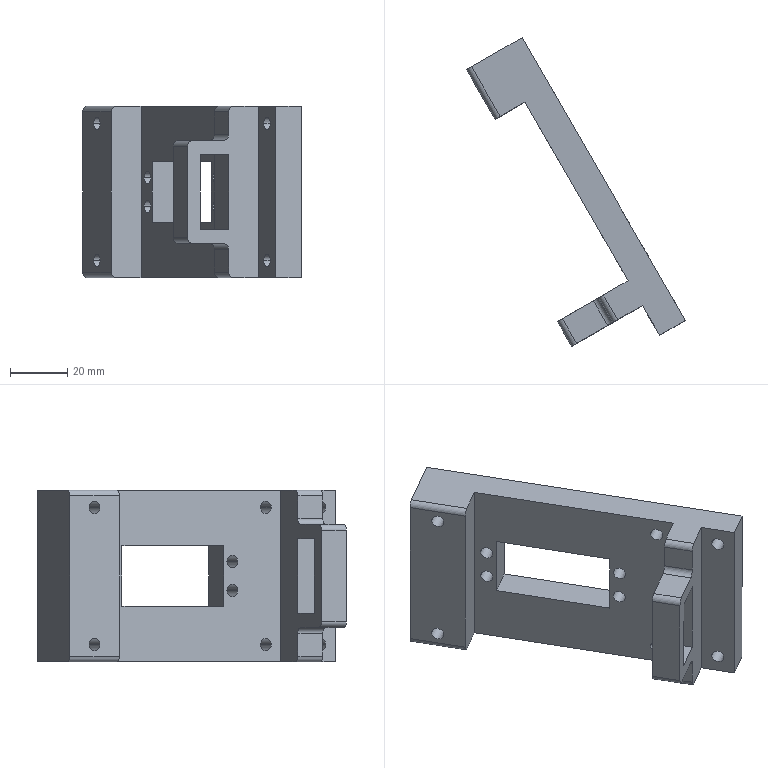Part | SolidWorks | features ICE 7, Fillet 4, Cut 2, Extrusion 1 | 1 solid | 52 faces | box 76.392 x 107.781 x 60 mm | volume 84689 mm3 | cylinder 28 | plane 24 | commonest cylinder face diameters 4.4 x20 4 x8